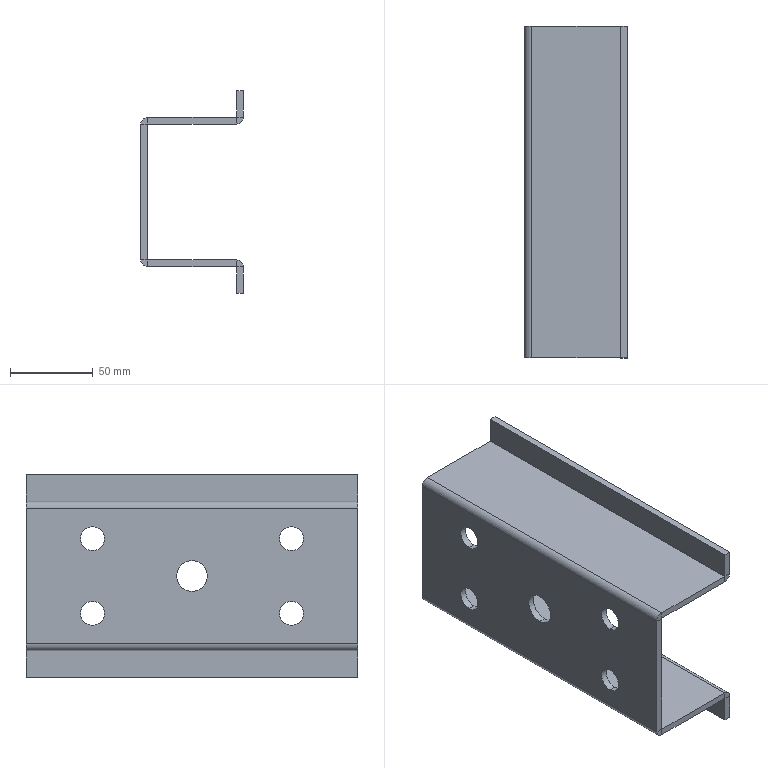Part | SolidWorks | features EdgeFlange 1, FlatPattern 1, ICE 1, SMBaseFlange 1, SheetMetal 1 | 1 solid | 48 faces | box 62 x 200 x 122 mm | volume 183661 mm3 | plane 30 | cylinder 18 | commonest cylinder face diameters 14.5 x8 0.4 x4 8.4 x4 18.5 x2
STEP:
#1=CARTESIAN_POINT('',(0.,0.,-9.25));
#2=VERTEX_POINT('',#1);
#3=CARTESIAN_POINT('',(0.,0.,9.25));
#4=VERTEX_POINT('',#3);
#5=CARTESIAN_POINT('',(0.,0.,0.));
#6=DIRECTION('',(-1.,0.,0.));
#7=DIRECTION('',(0.,0.,1.));
#8=AXIS2_PLACEMENT_3D('',#5,#6,#7);
#9=CIRCLE('',#8,9.25);
#10=EDGE_CURVE('',#2,#4,#9,.T.);
#11=ORIENTED_EDGE('',*,*,#10,.T.);
#12=CARTESIAN_POINT('',(4.,0.,9.25));
#13=VERTEX_POINT('',#12);
#14=CARTESIAN_POINT('',(-6.,0.,9.25));
#15=DIRECTION('',(1.,0.,0.));
#16=VECTOR('',#15,1000.);
#17=LINE('',#14,#16);
#18=EDGE_CURVE('',#4,#13,#17,.T.);
#19=ORIENTED_EDGE('',*,*,#18,.T.);
#20=CARTESIAN_POINT('',(4.,0.,-9.25));
#21=VERTEX_POINT('',#20);
#22=CARTESIAN_POINT('',(4.,0.,0.));
#23=DIRECTION('',(1.,0.,0.));
#24=DIRECTION('',(0.,0.,-1.));
#25=AXIS2_PLACEMENT_3D('',#22,#23,#24);
#26=CIRCLE('',#25,9.25);
#27=EDGE_CURVE('',#13,#21,#26,.T.);
#28=ORIENTED_EDGE('',*,*,#27,.T.);
#29=CARTESIAN_POINT('',(-6.,0.,-9.25));
#30=DIRECTION('',(1.,0.,0.));
#31=VECTOR('',#30,1000.);
#32=LINE('',#29,#31);
#33=EDGE_CURVE('',#2,#21,#32,.T.);
#34=ORIENTED_EDGE('',*,*,#33,.F.);
#35=EDGE_LOOP('',(#11,#19,#28,#34));
#36=FACE_OUTER_BOUND('',#35,.T.);
#37=CARTESIAN_POINT('',(-6.,0.,0.));
#38=DIRECTION('',(1.,0.,0.));
#39=DIRECTION('',(0.,0.,-1.));
#40=AXIS2_PLACEMENT_3D('',#37,#38,#39);
#41=CYLINDRICAL_SURFACE('',#40,9.25);
#42=ADVANCED_FACE('',(#36),#41,.F.);
#43=CARTESIAN_POINT('',(0.,-60.,-29.75));
#44=VERTEX_POINT('',#43);
#45=CARTESIAN_POINT('',(0.,-60.,-15.25));
#46=VERTEX_POINT('',#45);
#47=CARTESIAN_POINT('',(0.,-60.,-22.5));
#48=DIRECTION('',(-1.,0.,0.));
#49=DIRECTION('',(0.,0.,1.));
#50=AXIS2_PLACEMENT_3D('',#47,#48,#49);
#51=CIRCLE('',#50,7.25);
#52=EDGE_CURVE('',#44,#46,#51,.T.);
#53=ORIENTED_EDGE('',*,*,#52,.T.);
#54=CARTESIAN_POINT('',(4.,-60.,-15.25));
#55=VERTEX_POINT('',#54);
#56=CARTESIAN_POINT('',(-6.,-60.,-15.25));
#57=DIRECTION('',(1.,0.,0.));
#58=VECTOR('',#57,1000.);
#59=LINE('',#56,#58);
#60=EDGE_CURVE('',#46,#55,#59,.T.);
#61=ORIENTED_EDGE('',*,*,#60,.T.);
#62=CARTESIAN_POINT('',(4.,-60.,-29.75));
#63=VERTEX_POINT('',#62);
#64=CARTESIAN_POINT('',(4.,-60.,-22.5));
#65=DIRECTION('',(1.,0.,0.));
#66=DIRECTION('',(0.,0.,-1.));
#67=AXIS2_PLACEMENT_3D('',#64,#65,#66);
#68=CIRCLE('',#67,7.25);
#69=EDGE_CURVE('',#55,#63,#68,.T.);
#70=ORIENTED_EDGE('',*,*,#69,.T.);
#71=CARTESIAN_POINT('',(-6.,-60.,-29.75));
#72=DIRECTION('',(1.,0.,0.));
#73=VECTOR('',#72,1000.);
#74=LINE('',#71,#73);
#75=EDGE_CURVE('',#44,#63,#74,.T.);
#76=ORIENTED_EDGE('',*,*,#75,.F.);
#77=EDGE_LOOP('',(#53,#61,#70,#76));
#78=FACE_OUTER_BOUND('',#77,.T.);
#79=CARTESIAN_POINT('',(-6.,-60.,-22.5));
#80=DIRECTION('',(1.,0.,0.));
#81=DIRECTION('',(0.,0.,-1.));
#82=AXIS2_PLACEMENT_3D('',#79,#80,#81);
#83=CYLINDRICAL_SURFACE('',#82,7.25);
#84=ADVANCED_FACE('',(#78),#83,.F.);
#85=CARTESIAN_POINT('',(0.,-60.,15.25));
#86=VERTEX_POINT('',#85);
#87=CARTESIAN_POINT('',(0.,-60.,29.75));
#88=VERTEX_POINT('',#87);
#89=CARTESIAN_POINT('',(0.,-60.,22.5));
#90=DIRECTION('',(-1.,0.,0.));
#91=DIRECTION('',(0.,0.,1.));
#92=AXIS2_PLACEMENT_3D('',#89,#90,#91);
#93=CIRCLE('',#92,7.25);
#94=EDGE_CURVE('',#86,#88,#93,.T.);
#95=ORIENTED_EDGE('',*,*,#94,.T.);
#96=CARTESIAN_POINT('',(4.,-60.,29.75));
#97=VERTEX_POINT('',#96);
#98=CARTESIAN_POINT('',(-6.,-60.,29.75));
#99=DIRECTION('',(1.,0.,0.));
#100=VECTOR('',#99,1000.);
#101=LINE('',#98,#100);
#102=EDGE_CURVE('',#88,#97,#101,.T.);
#103=ORIENTED_EDGE('',*,*,#102,.T.);
#104=CARTESIAN_POINT('',(4.,-60.,15.25));
#105=VERTEX_POINT('',#104);
#106=CARTESIAN_POINT('',(4.,-60.,22.5));
#107=DIRECTION('',(1.,0.,0.));
#108=DIRECTION('',(0.,0.,-1.));
#109=AXIS2_PLACEMENT_3D('',#106,#107,#108);
#110=CIRCLE('',#109,7.25);
#111=EDGE_CURVE('',#97,#105,#110,.T.);
#112=ORIENTED_EDGE('',*,*,#111,.T.);
#113=CARTESIAN_POINT('',(-6.,-60.,15.25));
#114=DIRECTION('',(1.,0.,0.));
#115=VECTOR('',#114,1000.);
#116=LINE('',#113,#115);
#117=EDGE_CURVE('',#86,#105,#116,.T.);
#118=ORIENTED_EDGE('',*,*,#117,.F.);
#119=EDGE_LOOP('',(#95,#103,#112,#118));
#120=FACE_OUTER_BOUND('',#119,.T.);
#121=CARTESIAN_POINT('',(-6.,-60.,22.5));
#122=DIRECTION('',(1.,0.,0.));
#123=DIRECTION('',(0.,0.,-1.));
#124=AXIS2_PLACEMENT_3D('',#121,#122,#123);
#125=CYLINDRICAL_SURFACE('',#124,7.25);
#126=ADVANCED_FACE('',(#120),#125,.F.);
#127=CARTESIAN_POINT('',(0.,60.,15.25));
#128=VERTEX_POINT('',#127);
#129=CARTESIAN_POINT('',(0.,60.,29.75));
#130=VERTEX_POINT('',#129);
#131=CARTESIAN_POINT('',(0.,60.,22.5));
#132=DIRECTION('',(-1.,0.,0.));
#133=DIRECTION('',(0.,0.,1.));
#134=AXIS2_PLACEMENT_3D('',#131,#132,#133);
#135=CIRCLE('',#134,7.25);
#136=EDGE_CURVE('',#128,#130,#135,.T.);
#137=ORIENTED_EDGE('',*,*,#136,.T.);
#138=CARTESIAN_POINT('',(4.,60.,29.75));
#139=VERTEX_POINT('',#138);
#140=CARTESIAN_POINT('',(-6.,60.,29.75));
#141=DIRECTION('',(1.,0.,0.));
#142=VECTOR('',#141,1000.);
#143=LINE('',#140,#142);
#144=EDGE_CURVE('',#130,#139,#143,.T.);
#145=ORIENTED_EDGE('',*,*,#144,.T.);
#146=CARTESIAN_POINT('',(4.,60.,15.25));
#147=VERTEX_POINT('',#146);
#148=CARTESIAN_POINT('',(4.,60.,22.5));
#149=DIRECTION('',(1.,0.,0.));
#150=DIRECTION('',(0.,0.,-1.));
#151=AXIS2_PLACEMENT_3D('',#148,#149,#150);
#152=CIRCLE('',#151,7.25);
#153=EDGE_CURVE('',#139,#147,#152,.T.);
#154=ORIENTED_EDGE('',*,*,#153,.T.);
#155=CARTESIAN_POINT('',(-6.,60.,15.25));
#156=DIRECTION('',(1.,0.,0.));
#157=VECTOR('',#156,1000.);
#158=LINE('',#155,#157);
#159=EDGE_CURVE('',#128,#147,#158,.T.);
#160=ORIENTED_EDGE('',*,*,#159,.F.);
#161=EDGE_LOOP('',(#137,#145,#154,#160));
#162=FACE_OUTER_BOUND('',#161,.T.);
#163=CARTESIAN_POINT('',(-6.,60.,22.5));
#164=DIRECTION('',(1.,0.,0.));
#165=DIRECTION('',(0.,0.,-1.));
#166=AXIS2_PLACEMENT_3D('',#163,#164,#165);
#167=CYLINDRICAL_SURFACE('',#166,7.25);
#168=ADVANCED_FACE('',(#162),#167,.F.);
#169=CARTESIAN_POINT('',(0.,60.,-29.75));
#170=VERTEX_POINT('',#169);
#171=CARTESIAN_POINT('',(0.,60.,-15.25));
#172=VERTEX_POINT('',#171);
#173=CARTESIAN_POINT('',(0.,60.,-22.5));
#174=DIRECTION('',(-1.,0.,0.));
#175=DIRECTION('',(0.,0.,1.));
#176=AXIS2_PLACEMENT_3D('',#173,#174,#175);
#177=CIRCLE('',#176,7.25);
#178=EDGE_CURVE('',#170,#172,#177,.T.);
#179=ORIENTED_EDGE('',*,*,#178,.T.);
#180=CARTESIAN_POINT('',(4.,60.,-15.25));
#181=VERTEX_POINT('',#180);
#182=CARTESIAN_POINT('',(-6.,60.,-15.25));
#183=DIRECTION('',(1.,0.,0.));
#184=VECTOR('',#183,1000.);
#185=LINE('',#182,#184);
#186=EDGE_CURVE('',#172,#181,#185,.T.);
#187=ORIENTED_EDGE('',*,*,#186,.T.);
#188=CARTESIAN_POINT('',(4.,60.,-29.75));
#189=VERTEX_POINT('',#188);
#190=CARTESIAN_POINT('',(4.,60.,-22.5));
#191=DIRECTION('',(1.,0.,0.));
#192=DIRECTION('',(0.,0.,-1.));
#193=AXIS2_PLACEMENT_3D('',#190,#191,#192);
#194=CIRCLE('',#193,7.25);
#195=EDGE_CURVE('',#181,#189,#194,.T.);
#196=ORIENTED_EDGE('',*,*,#195,.T.);
#197=CARTESIAN_POINT('',(-6.,60.,-29.75));
#198=DIRECTION('',(1.,0.,0.));
#199=VECTOR('',#198,1000.);
#200=LINE('',#197,#199);
#201=EDGE_CURVE('',#170,#189,#200,.T.);
#202=ORIENTED_EDGE('',*,*,#201,.F.);
#203=EDGE_LOOP('',(#179,#187,#196,#202));
#204=FACE_OUTER_BOUND('',#203,.T.);
#205=CARTESIAN_POINT('',(-6.,60.,-22.5));
#206=DIRECTION('',(1.,0.,0.));
#207=DIRECTION('',(0.,0.,-1.));
#208=AXIS2_PLACEMENT_3D('',#205,#206,#207);
#209=CYLINDRICAL_SURFACE('',#208,7.25);
#210=ADVANCED_FACE('',(#204),#209,.F.);
#211=CARTESIAN_POINT('',(57.8,-100.,45.));
#212=VERTEX_POINT('',#211);
#213=CARTESIAN_POINT('',(4.2,-100.,45.));
#214=VERTEX_POINT('',#213);
#215=CARTESIAN_POINT('',(0.,-100.,45.));
#216=DIRECTION('',(-1.,0.,0.));
#217=VECTOR('',#216,1000.);
#218=LINE('',#215,#217);
#219=EDGE_CURVE('',#212,#214,#218,.T.);
#220=ORIENTED_EDGE('',*,*,#219,.F.);
#221=CARTESIAN_POINT('',(57.8,100.,45.));
#222=VERTEX_POINT('',#221);
#223=CARTESIAN_POINT('',(57.8,100.,45.));
#224=DIRECTION('',(0.,-1.,0.));
#225=VECTOR('',#224,1000.);
#226=LINE('',#223,#225);
#227=EDGE_CURVE('',#222,#212,#226,.T.);
#228=ORIENTED_EDGE('',*,*,#227,.F.);
#229=CARTESIAN_POINT('',(4.2,100.,45.));
#230=VERTEX_POINT('',#229);
#231=CARTESIAN_POINT('',(0.,100.,45.));
#232=DIRECTION('',(-1.,0.,0.));
#233=VECTOR('',#232,1000.);
#234=LINE('',#231,#233);
#235=EDGE_CURVE('',#222,#230,#234,.T.);
#236=ORIENTED_EDGE('',*,*,#235,.T.);
#237=CARTESIAN_POINT('',(4.2,100.,45.));
#238=DIRECTION('',(0.,-1.,0.));
#239=VECTOR('',#238,1000.);
#240=LINE('',#237,#239);
#241=EDGE_CURVE('',#230,#214,#240,.T.);
#242=ORIENTED_EDGE('',*,*,#241,.T.);
#243=EDGE_LOOP('',(#220,#228,#236,#242));
#244=FACE_OUTER_BOUND('',#243,.T.);
#245=CARTESIAN_POINT('',(0.,100.,45.));
#246=DIRECTION('',(0.,0.,1.));
#247=DIRECTION('',(1.,0.,0.));
#248=AXIS2_PLACEMENT_3D('',#245,#246,#247);
#249=PLANE('',#248);
#250=ADVANCED_FACE('',(#244),#249,.T.);
#251=CARTESIAN_POINT('',(57.8,100.,41.));
#252=VERTEX_POINT('',#251);
#253=CARTESIAN_POINT('',(57.8,-100.,41.));
#254=VERTEX_POINT('',#253);
#255=CARTESIAN_POINT('',(57.8,100.,41.));
#256=DIRECTION('',(0.,-1.,0.));
#257=VECTOR('',#256,1000.);
#258=LINE('',#255,#257);
#259=EDGE_CURVE('',#252,#254,#258,.T.);
#260=ORIENTED_EDGE('',*,*,#259,.T.);
#261=CARTESIAN_POINT('',(4.2,-100.,41.));
#262=VERTEX_POINT('',#261);
#263=CARTESIAN_POINT('',(0.,-100.,41.));
#264=DIRECTION('',(-1.,0.,0.));
#265=VECTOR('',#264,1000.);
#266=LINE('',#263,#265);
#267=EDGE_CURVE('',#254,#262,#266,.T.);
#268=ORIENTED_EDGE('',*,*,#267,.T.);
#269=CARTESIAN_POINT('',(4.2,100.,41.));
#270=VERTEX_POINT('',#269);
#271=CARTESIAN_POINT('',(4.2,100.,41.));
#272=DIRECTION('',(0.,-1.,0.));
#273=VECTOR('',#272,1000.);
#274=LINE('',#271,#273);
#275=EDGE_CURVE('',#270,#262,#274,.T.);
#276=ORIENTED_EDGE('',*,*,#275,.F.);
#277=CARTESIAN_POINT('',(0.,100.,41.));
#278=DIRECTION('',(-1.,0.,0.));
#279=VECTOR('',#278,1000.);
#280=LINE('',#277,#279);
#281=EDGE_CURVE('',#252,#270,#280,.T.);
#282=ORIENTED_EDGE('',*,*,#281,.F.);
#283=EDGE_LOOP('',(#260,#268,#276,#282));
#284=FACE_OUTER_BOUND('',#283,.T.);
#285=CARTESIAN_POINT('',(0.,100.,41.));
#286=DIRECTION('',(0.,0.,1.));
#287=DIRECTION('',(1.,0.,0.));
#288=AXIS2_PLACEMENT_3D('',#285,#286,#287);
#289=PLANE('',#288);
#290=ADVANCED_FACE('',(#284),#289,.F.);
#291=ORIENTED_EDGE('',*,*,#235,.F.);
#292=CARTESIAN_POINT('',(57.8,100.,45.));
#293=DIRECTION('',(0.,0.,-1.));
#294=VECTOR('',#293,1000.);
#295=LINE('',#292,#294);
#296=EDGE_CURVE('',#222,#252,#295,.T.);
#297=ORIENTED_EDGE('',*,*,#296,.T.);
#298=ORIENTED_EDGE('',*,*,#281,.T.);
#299=CARTESIAN_POINT('',(4.2,100.,41.));
#300=DIRECTION('',(0.,0.,1.));
#301=VECTOR('',#300,1000.);
#302=LINE('',#299,#301);
#303=EDGE_CURVE('',#270,#230,#302,.T.);
#304=ORIENTED_EDGE('',*,*,#303,.T.);
#305=EDGE_LOOP('',(#291,#297,#298,#304));
#306=FACE_OUTER_BOUND('',#305,.T.);
#307=CARTESIAN_POINT('',(4.2,100.,-40.8));
#308=DIRECTION('',(0.,1.,0.));
#309=DIRECTION('',(1.,0.,0.));
#310=AXIS2_PLACEMENT_3D('',#307,#308,#309);
#311=PLANE('',#310);
#312=ADVANCED_FACE('',(#306),#311,.T.);
#313=CARTESIAN_POINT('',(57.8,-100.,-41.));
#314=VERTEX_POINT('',#313);
#315=CARTESIAN_POINT('',(57.8,100.,-41.));
#316=VERTEX_POINT('',#315);
#317=CARTESIAN_POINT('',(57.8,-100.,-41.));
#318=DIRECTION('',(0.,1.,0.));
#319=VECTOR('',#318,1000.);
#320=LINE('',#317,#319);
#321=EDGE_CURVE('',#314,#316,#320,.T.);
#322=ORIENTED_EDGE('',*,*,#321,.T.);
#323=CARTESIAN_POINT('',(4.2,100.,-41.));
#324=VERTEX_POINT('',#323);
#325=CARTESIAN_POINT('',(0.,100.,-41.));
#326=DIRECTION('',(1.,0.,0.));
#327=VECTOR('',#326,1000.);
#328=LINE('',#325,#327);
#329=EDGE_CURVE('',#324,#316,#328,.T.);
#330=ORIENTED_EDGE('',*,*,#329,.F.);
#331=CARTESIAN_POINT('',(4.2,-100.,-41.));
#332=VERTEX_POINT('',#331);
#333=CARTESIAN_POINT('',(4.2,100.,-41.));
#334=DIRECTION('',(0.,-1.,0.));
#335=VECTOR('',#334,1000.);
#336=LINE('',#333,#335);
#337=EDGE_CURVE('',#324,#332,#336,.T.);
#338=ORIENTED_EDGE('',*,*,#337,.T.);
#339=CARTESIAN_POINT('',(0.,-100.,-41.));
#340=DIRECTION('',(1.,0.,0.));
#341=VECTOR('',#340,1000.);
#342=LINE('',#339,#341);
#343=EDGE_CURVE('',#332,#314,#342,.T.);
#344=ORIENTED_EDGE('',*,*,#343,.T.);
#345=EDGE_LOOP('',(#322,#330,#338,#344));
#346=FACE_OUTER_BOUND('',#345,.T.);
#347=CARTESIAN_POINT('',(0.,100.,-41.));
#348=DIRECTION('',(0.,0.,-1.));
#349=DIRECTION('',(-1.,0.,0.));
#350=AXIS2_PLACEMENT_3D('',#347,#348,#349);
#351=PLANE('',#350);
#352=ADVANCED_FACE('',(#346),#351,.F.);
#353=CARTESIAN_POINT('',(4.2,100.,-45.));
#354=VERTEX_POINT('',#353);
#355=CARTESIAN_POINT('',(57.8,100.,-45.));
#356=VERTEX_POINT('',#355);
#357=CARTESIAN_POINT('',(0.,100.,-45.));
#358=DIRECTION('',(1.,0.,0.));
#359=VECTOR('',#358,1000.);
#360=LINE('',#357,#359);
#361=EDGE_CURVE('',#354,#356,#360,.T.);
#362=ORIENTED_EDGE('',*,*,#361,.T.);
#363=CARTESIAN_POINT('',(57.8,-100.,-45.));
#364=VERTEX_POINT('',#363);
#365=CARTESIAN_POINT('',(57.8,-100.,-45.));
#366=DIRECTION('',(0.,1.,0.));
#367=VECTOR('',#366,1000.);
#368=LINE('',#365,#367);
#369=EDGE_CURVE('',#364,#356,#368,.T.);
#370=ORIENTED_EDGE('',*,*,#369,.F.);
#371=CARTESIAN_POINT('',(4.2,-100.,-45.));
#372=VERTEX_POINT('',#371);
#373=CARTESIAN_POINT('',(0.,-100.,-45.));
#374=DIRECTION('',(1.,0.,0.));
#375=VECTOR('',#374,1000.);
#376=LINE('',#373,#375);
#377=EDGE_CURVE('',#372,#364,#376,.T.);
#378=ORIENTED_EDGE('',*,*,#377,.F.);
#379=CARTESIAN_POINT('',(4.2,100.,-45.));
#380=DIRECTION('',(0.,-1.,0.));
#381=VECTOR('',#380,1000.);
#382=LINE('',#379,#381);
#383=EDGE_CURVE('',#354,#372,#382,.T.);
#384=ORIENTED_EDGE('',*,*,#383,.F.);
#385=EDGE_LOOP('',(#362,#370,#378,#384));
#386=FACE_OUTER_BOUND('',#385,.T.);
#387=CARTESIAN_POINT('',(0.,100.,-45.));
#388=DIRECTION('',(0.,0.,-1.));
#389=DIRECTION('',(-1.,0.,0.));
#390=AXIS2_PLACEMENT_3D('',#387,#388,#389);
#391=PLANE('',#390);
#392=ADVANCED_FACE('',(#386),#391,.T.);
#393=CARTESIAN_POINT('',(57.8,-100.,-45.));
#394=DIRECTION('',(0.,0.,1.));
#395=VECTOR('',#394,1000.);
#396=LINE('',#393,#395);
#397=EDGE_CURVE('',#364,#314,#396,.T.);
#398=ORIENTED_EDGE('',*,*,#397,.T.);
#399=ORIENTED_EDGE('',*,*,#343,.F.);
#400=CARTESIAN_POINT('',(4.2,-100.,-41.));
#401=DIRECTION('',(0.,0.,-1.));
#402=VECTOR('',#401,1000.);
#403=LINE('',#400,#402);
#404=EDGE_CURVE('',#332,#372,#403,.T.);
#405=ORIENTED_EDGE('',*,*,#404,.T.);
#406=ORIENTED_EDGE('',*,*,#377,.T.);
#407=EDGE_LOOP('',(#398,#399,#405,#406));
#408=FACE_OUTER_BOUND('',#407,.T.);
#409=CARTESIAN_POINT('',(4.2,-100.,-40.8));
#410=DIRECTION('',(0.,1.,0.));
#411=DIRECTION('',(1.,0.,0.));
#412=AXIS2_PLACEMENT_3D('',#409,#410,#411);
#413=PLANE('',#412);
#414=ADVANCED_FACE('',(#408),#413,.F.);
#415=CARTESIAN_POINT('',(0.,100.,40.8));
#416=VERTEX_POINT('',#415);
#417=CARTESIAN_POINT('',(4.,100.,40.8));
#418=VERTEX_POINT('',#417);
#419=CARTESIAN_POINT('',(0.,100.,40.8));
#420=DIRECTION('',(1.,0.,0.));
#421=VECTOR('',#420,1000.);
#422=LINE('',#419,#421);
#423=EDGE_CURVE('',#416,#418,#422,.T.);
#424=ORIENTED_EDGE('',*,*,#423,.F.);
#425=CARTESIAN_POINT('',(4.2,100.,40.8));
#426=DIRECTION('',(0.,-1.,0.));
#427=DIRECTION('',(0.,0.,1.));
#428=AXIS2_PLACEMENT_3D('',#425,#426,#427);
#429=CIRCLE('',#428,4.2);
#430=EDGE_CURVE('',#230,#416,#429,.T.);
#431=ORIENTED_EDGE('',*,*,#430,.F.);
#432=ORIENTED_EDGE('',*,*,#303,.F.);
#433=CARTESIAN_POINT('',(4.2,100.,40.8));
#434=DIRECTION('',(0.,-1.,0.));
#435=DIRECTION('',(1.,0.,0.));
#436=AXIS2_PLACEMENT_3D('',#433,#434,#435);
#437=CIRCLE('',#436,0.2);
#438=EDGE_CURVE('',#270,#418,#437,.T.);
#439=ORIENTED_EDGE('',*,*,#438,.T.);
#440=EDGE_LOOP('',(#424,#431,#432,#439));
#441=FACE_OUTER_BOUND('',#440,.T.);
#442=CARTESIAN_POINT('',(0.,100.,40.8));
#443=DIRECTION('',(0.,1.,0.));
#444=DIRECTION('',(0.,0.,1.));
#445=AXIS2_PLACEMENT_3D('',#442,#443,#444);
#446=PLANE('',#445);
#447=ADVANCED_FACE('',(#441),#446,.T.);
#448=CARTESIAN_POINT('',(0.,100.,-40.8));
#449=VERTEX_POINT('',#448);
#450=CARTESIAN_POINT('',(0.,100.,-45.));
#451=DIRECTION('',(0.,0.,-1.));
#452=VECTOR('',#451,1000.);
#453=LINE('',#450,#452);
#454=EDGE_CURVE('',#416,#449,#453,.T.);
#455=ORIENTED_EDGE('',*,*,#454,.F.);
#456=ORIENTED_EDGE('',*,*,#423,.T.);
#457=CARTESIAN_POINT('',(4.,100.,-40.8));
#458=VERTEX_POINT('',#457);
#459=CARTESIAN_POINT('',(4.,100.,-45.));
#460=DIRECTION('',(0.,0.,-1.));
#461=VECTOR('',#460,1000.);
#462=LINE('',#459,#461);
#463=EDGE_CURVE('',#418,#458,#462,.T.);
#464=ORIENTED_EDGE('',*,*,#463,.T.);
#465=CARTESIAN_POINT('',(4.,100.,-40.8));
#466=DIRECTION('',(-1.,0.,0.));
#467=VECTOR('',#466,1000.);
#468=LINE('',#465,#467);
#469=EDGE_CURVE('',#458,#449,#468,.T.);
#470=ORIENTED_EDGE('',*,*,#469,.T.);
#471=EDGE_LOOP('',(#455,#456,#464,#470));
#472=FACE_OUTER_BOUND('',#471,.T.);
#473=CARTESIAN_POINT('',(4.2,100.,41.));
#474=DIRECTION('',(0.,1.,0.));
#475=DIRECTION('',(0.,0.,1.));
#476=AXIS2_PLACEMENT_3D('',#473,#474,#475);
#477=PLANE('',#476);
#478=ADVANCED_FACE('',(#472),#477,.T.);
#479=CARTESIAN_POINT('',(4.2,-100.,45.));
#480=DIRECTION('',(0.,0.,-1.));
#481=VECTOR('',#480,1000.);
#482=LINE('',#479,#481);
#483=EDGE_CURVE('',#214,#262,#482,.T.);
#484=ORIENTED_EDGE('',*,*,#483,.F.);
#485=CARTESIAN_POINT('',(0.,-100.,40.8));
#486=VERTEX_POINT('',#485);
#487=CARTESIAN_POINT('',(4.2,-100.,40.8));
#488=DIRECTION('',(0.,-1.,0.));
#489=DIRECTION('',(0.,0.,1.));
#490=AXIS2_PLACEMENT_3D('',#487,#488,#489);
#491=CIRCLE('',#490,4.2);
#492=EDGE_CURVE('',#214,#486,#491,.T.);
#493=ORIENTED_EDGE('',*,*,#492,.T.);
#494=CARTESIAN_POINT('',(4.,-100.,40.8));
#495=VERTEX_POINT('',#494);
#496=CARTESIAN_POINT('',(4.,-100.,40.8));
#497=DIRECTION('',(-1.,0.,0.));
#498=VECTOR('',#497,1000.);
#499=LINE('',#496,#498);
#500=EDGE_CURVE('',#495,#486,#499,.T.);
#501=ORIENTED_EDGE('',*,*,#500,.F.);
#502=CARTESIAN_POINT('',(4.2,-100.,40.8));
#503=DIRECTION('',(0.,-1.,0.));
#504=DIRECTION('',(1.,0.,0.));
#505=AXIS2_PLACEMENT_3D('',#502,#503,#504);
#506=CIRCLE('',#505,0.2);
#507=EDGE_CURVE('',#262,#495,#506,.T.);
#508=ORIENTED_EDGE('',*,*,#507,.F.);
#509=EDGE_LOOP('',(#484,#493,#501,#508));
#510=FACE_OUTER_BOUND('',#509,.T.);
#511=CARTESIAN_POINT('',(4.2,-100.,45.));
#512=DIRECTION('',(0.,-1.,0.));
#513=DIRECTION('',(0.,0.,-1.));
#514=AXIS2_PLACEMENT_3D('',#511,#512,#513);
#515=PLANE('',#514);
#516=ADVANCED_FACE('',(#510),#515,.T.);
#517=CARTESIAN_POINT('',(57.8,-100.,45.));
#518=DIRECTION('',(0.,0.,-1.));
#519=VECTOR('',#518,1000.);
#520=LINE('',#517,#519);
#521=EDGE_CURVE('',#212,#254,#520,.T.);
#522=ORIENTED_EDGE('',*,*,#521,.F.);
#523=ORIENTED_EDGE('',*,*,#219,.T.);
#524=ORIENTED_EDGE('',*,*,#483,.T.);
#525=ORIENTED_EDGE('',*,*,#267,.F.);
#526=EDGE_LOOP('',(#522,#523,#524,#525));
#527=FACE_OUTER_BOUND('',#526,.T.);
#528=CARTESIAN_POINT('',(4.,-100.,40.8));
#529=DIRECTION('',(0.,-1.,0.));
#530=DIRECTION('',(0.,0.,-1.));
#531=AXIS2_PLACEMENT_3D('',#528,#529,#530);
#532=PLANE('',#531);
#533=ADVANCED_FACE('',(#527),#532,.T.);
#534=CARTESIAN_POINT('',(4.2,100.,-45.));
#535=DIRECTION('',(0.,0.,1.));
#536=VECTOR('',#535,1000.);
#537=LINE('',#534,#536);
#538=EDGE_CURVE('',#354,#324,#537,.T.);
#539=ORIENTED_EDGE('',*,*,#538,.F.);
#540=CARTESIAN_POINT('',(4.2,100.,-40.8));
#541=DIRECTION('',(0.,-1.,0.));
#542=DIRECTION('',(0.,0.,1.));
#543=AXIS2_PLACEMENT_3D('',#540,#541,#542);
#544=CIRCLE('',#543,4.2);
#545=EDGE_CURVE('',#449,#354,#544,.T.);
#546=ORIENTED_EDGE('',*,*,#545,.F.);
#547=ORIENTED_EDGE('',*,*,#469,.F.);
#548=CARTESIAN_POINT('',(4.2,100.,-40.8));
#549=DIRECTION('',(0.,-1.,0.));
#550=DIRECTION('',(1.,0.,0.));
#551=AXIS2_PLACEMENT_3D('',#548,#549,#550);
#552=CIRCLE('',#551,0.2);
#553=EDGE_CURVE('',#458,#324,#552,.T.);
#554=ORIENTED_EDGE('',*,*,#553,.T.);
#555=EDGE_LOOP('',(#539,#546,#547,#554));
#556=FACE_OUTER_BOUND('',#555,.T.);
#557=CARTESIAN_POINT('',(4.2,100.,-45.));
#558=DIRECTION('',(0.,1.,0.));
#559=DIRECTION('',(0.,0.,1.));
#560=AXIS2_PLACEMENT_3D('',#557,#558,#559);
#561=PLANE('',#560);
#562=ADVANCED_FACE('',(#556),#561,.T.);
#563=CARTESIAN_POINT('',(57.8,100.,-45.));
#564=DIRECTION('',(0.,0.,1.));
#565=VECTOR('',#564,1000.);
#566=LINE('',#563,#565);
#567=EDGE_CURVE('',#356,#316,#566,.T.);
#568=ORIENTED_EDGE('',*,*,#567,.F.);
#569=ORIENTED_EDGE('',*,*,#361,.F.);
#570=ORIENTED_EDGE('',*,*,#538,.T.);
#571=ORIENTED_EDGE('',*,*,#329,.T.);
#572=EDGE_LOOP('',(#568,#569,#570,#571));
#573=FACE_OUTER_BOUND('',#572,.T.);
#574=CARTESIAN_POINT('',(4.,100.,-40.8));
#575=DIRECTION('',(0.,1.,0.));
#576=DIRECTION('',(0.,0.,1.));
#577=AXIS2_PLACEMENT_3D('',#574,#575,#576);
#578=PLANE('',#577);
#579=ADVANCED_FACE('',(#573),#578,.T.);
#580=CARTESIAN_POINT('',(0.,-100.,-40.8));
#581=VERTEX_POINT('',#580);
#582=CARTESIAN_POINT('',(4.,-100.,-40.8));
#583=VERTEX_POINT('',#582);
#584=CARTESIAN_POINT('',(0.,-100.,-40.8));
#585=DIRECTION('',(1.,0.,0.));
#586=VECTOR('',#585,1000.);
#587=LINE('',#584,#586);
#588=EDGE_CURVE('',#581,#583,#587,.T.);
#589=ORIENTED_EDGE('',*,*,#588,.F.);
#590=CARTESIAN_POINT('',(4.2,-100.,-40.8));
#591=DIRECTION('',(0.,-1.,0.));
#592=DIRECTION('',(0.,0.,1.));
#593=AXIS2_PLACEMENT_3D('',#590,#591,#592);
#594=CIRCLE('',#593,4.2);
#595=EDGE_CURVE('',#581,#372,#594,.T.);
#596=ORIENTED_EDGE('',*,*,#595,.T.);
#597=ORIENTED_EDGE('',*,*,#404,.F.);
#598=CARTESIAN_POINT('',(4.2,-100.,-40.8));
#599=DIRECTION('',(0.,-1.,0.));
#600=DIRECTION('',(1.,0.,0.));
#601=AXIS2_PLACEMENT_3D('',#598,#599,#600);
#602=CIRCLE('',#601,0.2);
#603=EDGE_CURVE('',#583,#332,#602,.T.);
#604=ORIENTED_EDGE('',*,*,#603,.F.);
#605=EDGE_LOOP('',(#589,#596,#597,#604));
#606=FACE_OUTER_BOUND('',#605,.T.);
#607=CARTESIAN_POINT('',(0.,-100.,-40.8));
#608=DIRECTION('',(0.,-1.,0.));
#609=DIRECTION('',(0.,0.,-1.));
#610=AXIS2_PLACEMENT_3D('',#607,#608,#609);
#611=PLANE('',#610);
#612=ADVANCED_FACE('',(#606),#611,.T.);
#613=CARTESIAN_POINT('',(0.,-100.,-45.));
#614=DIRECTION('',(0.,0.,-1.));
#615=VECTOR('',#614,1000.);
#616=LINE('',#613,#615);
#617=EDGE_CURVE('',#486,#581,#616,.T.);
#618=ORIENTED_EDGE('',*,*,#617,.T.);
#619=ORIENTED_EDGE('',*,*,#588,.T.);
#620=CARTESIAN_POINT('',(4.,-100.,-45.));
#621=DIRECTION('',(0.,0.,-1.));
#622=VECTOR('',#621,1000.);
#623=LINE('',#620,#622);
#624=EDGE_CURVE('',#495,#583,#623,.T.);
#625=ORIENTED_EDGE('',*,*,#624,.F.);
#626=ORIENTED_EDGE('',*,*,#500,.T.);
#627=EDGE_LOOP('',(#618,#619,#625,#626));
#628=FACE_OUTER_BOUND('',#627,.T.);
#629=CARTESIAN_POINT('',(4.2,-100.,-41.));
#630=DIRECTION('',(0.,-1.,0.));
#631=DIRECTION('',(0.,0.,-1.));
#632=AXIS2_PLACEMENT_3D('',#629,#630,#631);
#633=PLANE('',#632);
#634=ADVANCED_FACE('',(#628),#633,.T.);
#635=ORIENTED_EDGE('',*,*,#595,.F.);
#636=CARTESIAN_POINT('',(0.,100.,-40.8));
#637=DIRECTION('',(0.,-1.,0.));
#638=VECTOR('',#637,1000.);
#639=LINE('',#636,#638);
#640=EDGE_CURVE('',#449,#581,#639,.T.);
#641=ORIENTED_EDGE('',*,*,#640,.F.);
#642=ORIENTED_EDGE('',*,*,#545,.T.);
#643=ORIENTED_EDGE('',*,*,#383,.T.);
#644=EDGE_LOOP('',(#635,#641,#642,#643));
#645=FACE_OUTER_BOUND('',#644,.T.);
#646=CARTESIAN_POINT('',(4.2,100.,-40.8));
#647=DIRECTION('',(0.,-1.,0.));
#648=DIRECTION('',(0.,0.,-1.));
#649=AXIS2_PLACEMENT_3D('',#646,#647,#648);
#650=CYLINDRICAL_SURFACE('',#649,4.2);
#651=ADVANCED_FACE('',(#645),#650,.T.);
#652=ORIENTED_EDGE('',*,*,#10,.F.);
#653=CARTESIAN_POINT('',(0.,0.,0.));
#654=DIRECTION('',(-1.,0.,0.));
#655=DIRECTION('',(0.,0.,1.));
#656=AXIS2_PLACEMENT_3D('',#653,#654,#655);
#657=CIRCLE('',#656,9.25);
#658=EDGE_CURVE('',#4,#2,#657,.T.);
#659=ORIENTED_EDGE('',*,*,#658,.F.);
#660=EDGE_LOOP('',(#652,#659));
#661=FACE_BOUND('',#660,.T.);
#662=ORIENTED_EDGE('',*,*,#52,.F.);
#663=CARTESIAN_POINT('',(0.,-60.,-22.5));
#664=DIRECTION('',(-1.,0.,0.));
#665=DIRECTION('',(0.,0.,1.));
#666=AXIS2_PLACEMENT_3D('',#663,#664,#665);
#667=CIRCLE('',#666,7.25);
#668=EDGE_CURVE('',#46,#44,#667,.T.);
#669=ORIENTED_EDGE('',*,*,#668,.F.);
#670=EDGE_LOOP('',(#662,#669));
#671=FACE_BOUND('',#670,.T.);
#672=ORIENTED_EDGE('',*,*,#94,.F.);
#673=CARTESIAN_POINT('',(0.,-60.,22.5));
#674=DIRECTION('',(-1.,0.,0.));
#675=DIRECTION('',(0.,0.,1.));
#676=AXIS2_PLACEMENT_3D('',#673,#674,#675);
#677=CIRCLE('',#676,7.25);
#678=EDGE_CURVE('',#88,#86,#677,.T.);
#679=ORIENTED_EDGE('',*,*,#678,.F.);
#680=EDGE_LOOP('',(#672,#679));
#681=FACE_BOUND('',#680,.T.);
#682=ORIENTED_EDGE('',*,*,#136,.F.);
#683=CARTESIAN_POINT('',(0.,60.,22.5));
#684=DIRECTION('',(-1.,0.,0.));
#685=DIRECTION('',(0.,0.,1.));
#686=AXIS2_PLACEMENT_3D('',#683,#684,#685);
#687=CIRCLE('',#686,7.25);
#688=EDGE_CURVE('',#130,#128,#687,.T.);
#689=ORIENTED_EDGE('',*,*,#688,.F.);
#690=EDGE_LOOP('',(#682,#689));
#691=FACE_BOUND('',#690,.T.);
#692=ORIENTED_EDGE('',*,*,#178,.F.);
#693=CARTESIAN_POINT('',(0.,60.,-22.5));
#694=DIRECTION('',(-1.,0.,0.));
#695=DIRECTION('',(0.,0.,1.));
#696=AXIS2_PLACEMENT_3D('',#693,#694,#695);
#697=CIRCLE('',#696,7.25);
#698=EDGE_CURVE('',#172,#170,#697,.T.);
#699=ORIENTED_EDGE('',*,*,#698,.F.);
#700=EDGE_LOOP('',(#692,#699));
#701=FACE_BOUND('',#700,.T.);
#702=ORIENTED_EDGE('',*,*,#617,.F.);
#703=CARTESIAN_POINT('',(0.,100.,40.8));
#704=DIRECTION('',(0.,-1.,0.));
#705=VECTOR('',#704,1000.);
#706=LINE('',#703,#705);
#707=EDGE_CURVE('',#416,#486,#706,.T.);
#708=ORIENTED_EDGE('',*,*,#707,.F.);
#709=ORIENTED_EDGE('',*,*,#454,.T.);
#710=ORIENTED_EDGE('',*,*,#640,.T.);
#711=EDGE_LOOP('',(#702,#708,#709,#710));
#712=FACE_OUTER_BOUND('',#711,.T.);
#713=CARTESIAN_POINT('',(0.,100.,-45.));
#714=DIRECTION('',(-1.,0.,0.));
#715=DIRECTION('',(0.,0.,1.));
#716=AXIS2_PLACEMENT_3D('',#713,#714,#715);
#717=PLANE('',#716);
#718=ADVANCED_FACE('',(#661,#671,#681,#691,#701,#712),#717,.T.);
#719=ORIENTED_EDGE('',*,*,#492,.F.);
#720=ORIENTED_EDGE('',*,*,#241,.F.);
#721=ORIENTED_EDGE('',*,*,#430,.T.);
#722=ORIENTED_EDGE('',*,*,#707,.T.);
#723=EDGE_LOOP('',(#719,#720,#721,#722));
#724=FACE_OUTER_BOUND('',#723,.T.);
#725=CARTESIAN_POINT('',(4.2,100.,40.8));
#726=DIRECTION('',(0.,-1.,0.));
#727=DIRECTION('',(0.,0.,-1.));
#728=AXIS2_PLACEMENT_3D('',#725,#726,#727);
#729=CYLINDRICAL_SURFACE('',#728,4.2);
#730=ADVANCED_FACE('',(#724),#729,.T.);
#731=ORIENTED_EDGE('',*,*,#507,.T.);
#732=CARTESIAN_POINT('',(4.,100.,40.8));
#733=DIRECTION('',(0.,-1.,0.));
#734=VECTOR('',#733,1000.);
#735=LINE('',#732,#734);
#736=EDGE_CURVE('',#418,#495,#735,.T.);
#737=ORIENTED_EDGE('',*,*,#736,.F.);
#738=ORIENTED_EDGE('',*,*,#438,.F.);
#739=ORIENTED_EDGE('',*,*,#275,.T.);
#740=EDGE_LOOP('',(#731,#737,#738,#739));
#741=FACE_OUTER_BOUND('',#740,.T.);
#742=CARTESIAN_POINT('',(4.2,100.,40.8));
#743=DIRECTION('',(0.,-1.,0.));
#744=DIRECTION('',(0.,0.,-1.));
#745=AXIS2_PLACEMENT_3D('',#742,#743,#744);
#746=CYLINDRICAL_SURFACE('',#745,0.2);
#747=ADVANCED_FACE('',(#741),#746,.F.);
#748=CARTESIAN_POINT('',(4.,0.,0.));
#749=DIRECTION('',(1.,0.,0.));
#750=DIRECTION('',(0.,0.,-1.));
#751=AXIS2_PLACEMENT_3D('',#748,#749,#750);
#752=CIRCLE('',#751,9.25);
#753=EDGE_CURVE('',#21,#13,#752,.T.);
#754=ORIENTED_EDGE('',*,*,#753,.F.);
#755=ORIENTED_EDGE('',*,*,#27,.F.);
#756=EDGE_LOOP('',(#754,#755));
#757=FACE_BOUND('',#756,.T.);
#758=CARTESIAN_POINT('',(4.,-60.,-22.5));
#759=DIRECTION('',(1.,0.,0.));
#760=DIRECTION('',(0.,0.,-1.));
#761=AXIS2_PLACEMENT_3D('',#758,#759,#760);
#762=CIRCLE('',#761,7.25);
#763=EDGE_CURVE('',#63,#55,#762,.T.);
#764=ORIENTED_EDGE('',*,*,#763,.F.);
#765=ORIENTED_EDGE('',*,*,#69,.F.);
#766=EDGE_LOOP('',(#764,#765));
#767=FACE_BOUND('',#766,.T.);
#768=CARTESIAN_POINT('',(4.,-60.,22.5));
#769=DIRECTION('',(1.,0.,0.));
#770=DIRECTION('',(0.,0.,-1.));
#771=AXIS2_PLACEMENT_3D('',#768,#769,#770);
#772=CIRCLE('',#771,7.25);
#773=EDGE_CURVE('',#105,#97,#772,.T.);
#774=ORIENTED_EDGE('',*,*,#773,.F.);
#775=ORIENTED_EDGE('',*,*,#111,.F.);
#776=EDGE_LOOP('',(#774,#775));
#777=FACE_BOUND('',#776,.T.);
#778=CARTESIAN_POINT('',(4.,60.,22.5));
#779=DIRECTION('',(1.,0.,0.));
#780=DIRECTION('',(0.,0.,-1.));
#781=AXIS2_PLACEMENT_3D('',#778,#779,#780);
#782=CIRCLE('',#781,7.25);
#783=EDGE_CURVE('',#147,#139,#782,.T.);
#784=ORIENTED_EDGE('',*,*,#783,.F.);
#785=ORIENTED_EDGE('',*,*,#153,.F.);
#786=EDGE_LOOP('',(#784,#785));
#787=FACE_BOUND('',#786,.T.);
#788=CARTESIAN_POINT('',(4.,60.,-22.5));
#789=DIRECTION('',(1.,0.,0.));
#790=DIRECTION('',(0.,0.,-1.));
#791=AXIS2_PLACEMENT_3D('',#788,#789,#790);
#792=CIRCLE('',#791,7.25);
#793=EDGE_CURVE('',#189,#181,#792,.T.);
#794=ORIENTED_EDGE('',*,*,#793,.F.);
#795=ORIENTED_EDGE('',*,*,#195,.F.);
#796=EDGE_LOOP('',(#794,#795));
#797=FACE_BOUND('',#796,.T.);
#798=ORIENTED_EDGE('',*,*,#624,.T.);
#799=CARTESIAN_POINT('',(4.,100.,-40.8));
#800=DIRECTION('',(0.,-1.,0.));
#801=VECTOR('',#800,1000.);
#802=LINE('',#799,#801);
#803=EDGE_CURVE('',#458,#583,#802,.T.);
#804=ORIENTED_EDGE('',*,*,#803,.F.);
#805=ORIENTED_EDGE('',*,*,#463,.F.);
#806=ORIENTED_EDGE('',*,*,#736,.T.);
#807=EDGE_LOOP('',(#798,#804,#805,#806));
#808=FACE_OUTER_BOUND('',#807,.T.);
#809=CARTESIAN_POINT('',(4.,100.,-45.));
#810=DIRECTION('',(-1.,0.,0.));
#811=DIRECTION('',(0.,0.,1.));
#812=AXIS2_PLACEMENT_3D('',#809,#810,#811);
#813=PLANE('',#812);
#814=ADVANCED_FACE('',(#757,#767,#777,#787,#797,#808),#813,.F.);
#815=ORIENTED_EDGE('',*,*,#603,.T.);
#816=ORIENTED_EDGE('',*,*,#337,.F.);
#817=ORIENTED_EDGE('',*,*,#553,.F.);
#818=ORIENTED_EDGE('',*,*,#803,.T.);
#819=EDGE_LOOP('',(#815,#816,#817,#818));
#820=FACE_OUTER_BOUND('',#819,.T.);
#821=CARTESIAN_POINT('',(4.2,100.,-40.8));
#822=DIRECTION('',(0.,-1.,0.));
#823=DIRECTION('',(0.,0.,-1.));
#824=AXIS2_PLACEMENT_3D('',#821,#822,#823);
#825=CYLINDRICAL_SURFACE('',#824,0.2);
#826=ADVANCED_FACE('',(#820),#825,.F.);
#827=CARTESIAN_POINT('',(58.,100.,-45.2));
#828=VERTEX_POINT('',#827);
#829=CARTESIAN_POINT('',(62.,100.,-45.2));
#830=VERTEX_POINT('',#829);
#831=CARTESIAN_POINT('',(62.,100.,-45.2));
#832=DIRECTION('',(1.,0.,0.));
#833=VECTOR('',#832,1000.);
#834=LINE('',#831,#833);
#835=EDGE_CURVE('',#828,#830,#834,.T.);
#836=ORIENTED_EDGE('',*,*,#835,.F.);
#837=CARTESIAN_POINT('',(57.8,100.,-45.2));
#838=DIRECTION('',(0.,1.,0.));
#839=DIRECTION('',(0.,0.,-1.));
#840=AXIS2_PLACEMENT_3D('',#837,#838,#839);
#841=CIRCLE('',#840,0.2);
#842=EDGE_CURVE('',#356,#828,#841,.T.);
#843=ORIENTED_EDGE('',*,*,#842,.F.);
#844=ORIENTED_EDGE('',*,*,#567,.T.);
#845=CARTESIAN_POINT('',(57.8,100.,-45.2));
#846=DIRECTION('',(0.,1.,0.));
#847=DIRECTION('',(0.,0.,-1.));
#848=AXIS2_PLACEMENT_3D('',#845,#846,#847);
#849=CIRCLE('',#848,4.2);
#850=EDGE_CURVE('',#316,#830,#849,.T.);
#851=ORIENTED_EDGE('',*,*,#850,.T.);
#852=EDGE_LOOP('',(#836,#843,#844,#851));
#853=FACE_OUTER_BOUND('',#852,.T.);
#854=CARTESIAN_POINT('',(57.8,100.,-45.2));
#855=DIRECTION('',(0.,1.,0.));
#856=DIRECTION('',(0.,0.,1.));
#857=AXIS2_PLACEMENT_3D('',#854,#855,#856);
#858=PLANE('',#857);
#859=ADVANCED_FACE('',(#853),#858,.T.);
#860=CARTESIAN_POINT('',(58.,-100.,-45.2));
#861=VERTEX_POINT('',#860);
#862=CARTESIAN_POINT('',(57.8,-100.,-45.2));
#863=DIRECTION('',(0.,-1.,0.));
#864=DIRECTION('',(0.,0.,-1.));
#865=AXIS2_PLACEMENT_3D('',#862,#863,#864);
#866=CIRCLE('',#865,0.2);
#867=EDGE_CURVE('',#861,#364,#866,.T.);
#868=ORIENTED_EDGE('',*,*,#867,.F.);
#869=CARTESIAN_POINT('',(62.,-100.,-45.2));
#870=VERTEX_POINT('',#869);
#871=CARTESIAN_POINT('',(58.,-100.,-45.2));
#872=DIRECTION('',(1.,0.,0.));
#873=VECTOR('',#872,1000.);
#874=LINE('',#871,#873);
#875=EDGE_CURVE('',#861,#870,#874,.T.);
#876=ORIENTED_EDGE('',*,*,#875,.T.);
#877=CARTESIAN_POINT('',(57.8,-100.,-45.2));
#878=DIRECTION('',(0.,-1.,0.));
#879=DIRECTION('',(0.,0.,-1.));
#880=AXIS2_PLACEMENT_3D('',#877,#878,#879);
#881=CIRCLE('',#880,4.2);
#882=EDGE_CURVE('',#870,#314,#881,.T.);
#883=ORIENTED_EDGE('',*,*,#882,.T.);
#884=ORIENTED_EDGE('',*,*,#397,.F.);
#885=EDGE_LOOP('',(#868,#876,#883,#884));
#886=FACE_OUTER_BOUND('',#885,.T.);
#887=CARTESIAN_POINT('',(57.8,-100.,-45.2));
#888=DIRECTION('',(0.,1.,0.));
#889=DIRECTION('',(0.,0.,1.));
#890=AXIS2_PLACEMENT_3D('',#887,#888,#889);
#891=PLANE('',#890);
#892=ADVANCED_FACE('',(#886),#891,.F.);
#893=ORIENTED_EDGE('',*,*,#321,.F.);
#894=ORIENTED_EDGE('',*,*,#882,.F.);
#895=CARTESIAN_POINT('',(62.,100.,-45.2));
#896=DIRECTION('',(0.,1.,0.));
#897=VECTOR('',#896,1000.);
#898=LINE('',#895,#897);
#899=EDGE_CURVE('',#870,#830,#898,.T.);
#900=ORIENTED_EDGE('',*,*,#899,.T.);
#901=ORIENTED_EDGE('',*,*,#850,.F.);
#902=EDGE_LOOP('',(#893,#894,#900,#901));
#903=FACE_OUTER_BOUND('',#902,.T.);
#904=CARTESIAN_POINT('',(57.8,-100.,-45.2));
#905=DIRECTION('',(0.,-1.,0.));
#906=DIRECTION('',(1.,0.,0.));
#907=AXIS2_PLACEMENT_3D('',#904,#905,#906);
#908=CYLINDRICAL_SURFACE('',#907,4.2);
#909=ADVANCED_FACE('',(#903),#908,.T.);
#910=ORIENTED_EDGE('',*,*,#369,.T.);
#911=ORIENTED_EDGE('',*,*,#842,.T.);
#912=CARTESIAN_POINT('',(58.,100.,-45.2));
#913=DIRECTION('',(0.,-1.,0.));
#914=VECTOR('',#913,1000.);
#915=LINE('',#912,#914);
#916=EDGE_CURVE('',#828,#861,#915,.T.);
#917=ORIENTED_EDGE('',*,*,#916,.T.);
#918=ORIENTED_EDGE('',*,*,#867,.T.);
#919=EDGE_LOOP('',(#910,#911,#917,#918));
#920=FACE_OUTER_BOUND('',#919,.T.);
#921=CARTESIAN_POINT('',(57.8,-100.,-45.2));
#922=DIRECTION('',(0.,-1.,0.));
#923=DIRECTION('',(1.,0.,0.));
#924=AXIS2_PLACEMENT_3D('',#921,#922,#923);
#925=CYLINDRICAL_SURFACE('',#924,0.2);
#926=ADVANCED_FACE('',(#920),#925,.F.);
#927=ORIENTED_EDGE('',*,*,#875,.F.);
#928=CARTESIAN_POINT('',(58.,-100.,-61.));
#929=VERTEX_POINT('',#928);
#930=CARTESIAN_POINT('',(58.,-100.,-61.));
#931=DIRECTION('',(0.,0.,-1.));
#932=VECTOR('',#931,1000.);
#933=LINE('',#930,#932);
#934=EDGE_CURVE('',#861,#929,#933,.T.);
#935=ORIENTED_EDGE('',*,*,#934,.T.);
#936=CARTESIAN_POINT('',(62.,-100.,-61.));
#937=VERTEX_POINT('',#936);
#938=CARTESIAN_POINT('',(62.,-100.,-61.));
#939=DIRECTION('',(-1.,0.,0.));
#940=VECTOR('',#939,1000.);
#941=LINE('',#938,#940);
#942=EDGE_CURVE('',#937,#929,#941,.T.);
#943=ORIENTED_EDGE('',*,*,#942,.F.);
#944=CARTESIAN_POINT('',(62.,-100.,0.));
#945=DIRECTION('',(0.,0.,-1.));
#946=VECTOR('',#945,1000.);
#947=LINE('',#944,#946);
#948=EDGE_CURVE('',#870,#937,#947,.T.);
#949=ORIENTED_EDGE('',*,*,#948,.F.);
#950=EDGE_LOOP('',(#927,#935,#943,#949));
#951=FACE_OUTER_BOUND('',#950,.T.);
#952=CARTESIAN_POINT('',(62.,-100.,-61.));
#953=DIRECTION('',(0.,1.,0.));
#954=DIRECTION('',(0.,0.,1.));
#955=AXIS2_PLACEMENT_3D('',#952,#953,#954);
#956=PLANE('',#955);
#957=ADVANCED_FACE('',(#951),#956,.F.);
#958=ORIENTED_EDGE('',*,*,#835,.T.);
#959=CARTESIAN_POINT('',(62.,100.,-61.));
#960=VERTEX_POINT('',#959);
#961=CARTESIAN_POINT('',(62.,100.,0.));
#962=DIRECTION('',(0.,0.,1.));
#963=VECTOR('',#962,1000.);
#964=LINE('',#961,#963);
#965=EDGE_CURVE('',#960,#830,#964,.T.);
#966=ORIENTED_EDGE('',*,*,#965,.F.);
#967=CARTESIAN_POINT('',(58.,100.,-61.));
#968=VERTEX_POINT('',#967);
#969=CARTESIAN_POINT('',(62.,100.,-61.));
#970=DIRECTION('',(-1.,0.,0.));
#971=VECTOR('',#970,1000.);
#972=LINE('',#969,#971);
#973=EDGE_CURVE('',#960,#968,#972,.T.);
#974=ORIENTED_EDGE('',*,*,#973,.T.);
#975=CARTESIAN_POINT('',(58.,100.,-45.));
#976=DIRECTION('',(0.,0.,1.));
#977=VECTOR('',#976,1000.);
#978=LINE('',#975,#977);
#979=EDGE_CURVE('',#968,#828,#978,.T.);
#980=ORIENTED_EDGE('',*,*,#979,.T.);
#981=EDGE_LOOP('',(#958,#966,#974,#980));
#982=FACE_OUTER_BOUND('',#981,.T.);
#983=CARTESIAN_POINT('',(62.,100.,-45.));
#984=DIRECTION('',(0.,-1.,0.));
#985=DIRECTION('',(0.,0.,-1.));
#986=AXIS2_PLACEMENT_3D('',#983,#984,#985);
#987=PLANE('',#986);
#988=ADVANCED_FACE('',(#982),#987,.F.);
#989=ORIENTED_EDGE('',*,*,#899,.F.);
#990=ORIENTED_EDGE('',*,*,#948,.T.);
#991=CARTESIAN_POINT('',(62.,0.,-61.));
#992=DIRECTION('',(0.,1.,0.));
#993=VECTOR('',#992,1000.);
#994=LINE('',#991,#993);
#995=EDGE_CURVE('',#937,#960,#994,.T.);
#996=ORIENTED_EDGE('',*,*,#995,.T.);
#997=ORIENTED_EDGE('',*,*,#965,.T.);
#998=EDGE_LOOP('',(#989,#990,#996,#997));
#999=FACE_OUTER_BOUND('',#998,.T.);
#1000=CARTESIAN_POINT('',(62.,0.,0.));
#1001=DIRECTION('',(-1.,0.,0.));
#1002=DIRECTION('',(0.,0.,1.));
#1003=AXIS2_PLACEMENT_3D('',#1000,#1001,#1002);
#1004=PLANE('',#1003);
#1005=ADVANCED_FACE('',(#999),#1004,.F.);
#1006=ORIENTED_EDGE('',*,*,#934,.F.);
#1007=ORIENTED_EDGE('',*,*,#916,.F.);
#1008=ORIENTED_EDGE('',*,*,#979,.F.);
#1009=CARTESIAN_POINT('',(58.,100.,-61.));
#1010=DIRECTION('',(0.,1.,0.));
#1011=VECTOR('',#1010,1000.);
#1012=LINE('',#1009,#1011);
#1013=EDGE_CURVE('',#929,#968,#1012,.T.);
#1014=ORIENTED_EDGE('',*,*,#1013,.F.);
#1015=EDGE_LOOP('',(#1006,#1007,#1008,#1014));
#1016=FACE_OUTER_BOUND('',#1015,.T.);
#1017=CARTESIAN_POINT('',(58.,0.,0.));
#1018=DIRECTION('',(-1.,0.,0.));
#1019=DIRECTION('',(0.,0.,1.));
#1020=AXIS2_PLACEMENT_3D('',#1017,#1018,#1019);
#1021=PLANE('',#1020);
#1022=ADVANCED_FACE('',(#1016),#1021,.T.);
#1023=ORIENTED_EDGE('',*,*,#1013,.T.);
#1024=ORIENTED_EDGE('',*,*,#973,.F.);
#1025=ORIENTED_EDGE('',*,*,#995,.F.);
#1026=ORIENTED_EDGE('',*,*,#942,.T.);
#1027=EDGE_LOOP('',(#1023,#1024,#1025,#1026));
#1028=FACE_OUTER_BOUND('',#1027,.T.);
#1029=CARTESIAN_POINT('',(62.,100.,-61.));
#1030=DIRECTION('',(0.,0.,1.));
#1031=DIRECTION('',(1.,0.,0.));
#1032=AXIS2_PLACEMENT_3D('',#1029,#1030,#1031);
#1033=PLANE('',#1032);
#1034=ADVANCED_FACE('',(#1028),#1033,.F.);
#1035=CARTESIAN_POINT('',(58.,-100.,45.2));
#1036=VERTEX_POINT('',#1035);
#1037=CARTESIAN_POINT('',(62.,-100.,45.2));
#1038=VERTEX_POINT('',#1037);
#1039=CARTESIAN_POINT('',(62.,-100.,45.2));
#1040=DIRECTION('',(1.,0.,0.));
#1041=VECTOR('',#1040,1000.);
#1042=LINE('',#1039,#1041);
#1043=EDGE_CURVE('',#1036,#1038,#1042,.T.);
#1044=ORIENTED_EDGE('',*,*,#1043,.F.);
#1045=CARTESIAN_POINT('',(57.8,-100.,45.2));
#1046=DIRECTION('',(0.,-1.,0.));
#1047=DIRECTION('',(0.,0.,1.));
#1048=AXIS2_PLACEMENT_3D('',#1045,#1046,#1047);
#1049=CIRCLE('',#1048,0.2);
#1050=EDGE_CURVE('',#212,#1036,#1049,.T.);
#1051=ORIENTED_EDGE('',*,*,#1050,.F.);
#1052=ORIENTED_EDGE('',*,*,#521,.T.);
#1053=CARTESIAN_POINT('',(57.8,-100.,45.2));
#1054=DIRECTION('',(0.,-1.,0.));
#1055=DIRECTION('',(0.,0.,1.));
#1056=AXIS2_PLACEMENT_3D('',#1053,#1054,#1055);
#1057=CIRCLE('',#1056,4.2);
#1058=EDGE_CURVE('',#254,#1038,#1057,.T.);
#1059=ORIENTED_EDGE('',*,*,#1058,.T.);
#1060=EDGE_LOOP('',(#1044,#1051,#1052,#1059));
#1061=FACE_OUTER_BOUND('',#1060,.T.);
#1062=CARTESIAN_POINT('',(57.8,-100.,45.2));
#1063=DIRECTION('',(0.,-1.,0.));
#1064=DIRECTION('',(0.,0.,-1.));
#1065=AXIS2_PLACEMENT_3D('',#1062,#1063,#1064);
#1066=PLANE('',#1065);
#1067=ADVANCED_FACE('',(#1061),#1066,.T.);
#1068=CARTESIAN_POINT('',(58.,100.,45.2));
#1069=VERTEX_POINT('',#1068);
#1070=CARTESIAN_POINT('',(57.8,100.,45.2));
#1071=DIRECTION('',(0.,1.,0.));
#1072=DIRECTION('',(0.,0.,1.));
#1073=AXIS2_PLACEMENT_3D('',#1070,#1071,#1072);
#1074=CIRCLE('',#1073,0.2);
#1075=EDGE_CURVE('',#1069,#222,#1074,.T.);
#1076=ORIENTED_EDGE('',*,*,#1075,.F.);
#1077=CARTESIAN_POINT('',(62.,100.,45.2));
#1078=VERTEX_POINT('',#1077);
#1079=CARTESIAN_POINT('',(58.,100.,45.2));
#1080=DIRECTION('',(1.,0.,0.));
#1081=VECTOR('',#1080,1000.);
#1082=LINE('',#1079,#1081);
#1083=EDGE_CURVE('',#1069,#1078,#1082,.T.);
#1084=ORIENTED_EDGE('',*,*,#1083,.T.);
#1085=CARTESIAN_POINT('',(57.8,100.,45.2));
#1086=DIRECTION('',(0.,1.,0.));
#1087=DIRECTION('',(0.,0.,1.));
#1088=AXIS2_PLACEMENT_3D('',#1085,#1086,#1087);
#1089=CIRCLE('',#1088,4.2);
#1090=EDGE_CURVE('',#1078,#252,#1089,.T.);
#1091=ORIENTED_EDGE('',*,*,#1090,.T.);
#1092=ORIENTED_EDGE('',*,*,#296,.F.);
#1093=EDGE_LOOP('',(#1076,#1084,#1091,#1092));
#1094=FACE_OUTER_BOUND('',#1093,.T.);
#1095=CARTESIAN_POINT('',(57.8,100.,45.2));
#1096=DIRECTION('',(0.,-1.,0.));
#1097=DIRECTION('',(0.,0.,-1.));
#1098=AXIS2_PLACEMENT_3D('',#1095,#1096,#1097);
#1099=PLANE('',#1098);
#1100=ADVANCED_FACE('',(#1094),#1099,.F.);
#1101=ORIENTED_EDGE('',*,*,#259,.F.);
#1102=ORIENTED_EDGE('',*,*,#1090,.F.);
#1103=CARTESIAN_POINT('',(62.,-100.,45.2));
#1104=DIRECTION('',(0.,-1.,0.));
#1105=VECTOR('',#1104,1000.);
#1106=LINE('',#1103,#1105);
#1107=EDGE_CURVE('',#1078,#1038,#1106,.T.);
#1108=ORIENTED_EDGE('',*,*,#1107,.T.);
#1109=ORIENTED_EDGE('',*,*,#1058,.F.);
#1110=EDGE_LOOP('',(#1101,#1102,#1108,#1109));
#1111=FACE_OUTER_BOUND('',#1110,.T.);
#1112=CARTESIAN_POINT('',(57.8,100.,45.2));
#1113=DIRECTION('',(0.,1.,0.));
#1114=DIRECTION('',(1.,0.,0.));
#1115=AXIS2_PLACEMENT_3D('',#1112,#1113,#1114);
#1116=CYLINDRICAL_SURFACE('',#1115,4.2);
#1117=ADVANCED_FACE('',(#1111),#1116,.T.);
#1118=ORIENTED_EDGE('',*,*,#227,.T.);
#1119=ORIENTED_EDGE('',*,*,#1050,.T.);
#1120=CARTESIAN_POINT('',(58.,-100.,45.2));
#1121=DIRECTION('',(0.,1.,0.));
#1122=VECTOR('',#1121,1000.);
#1123=LINE('',#1120,#1122);
#1124=EDGE_CURVE('',#1036,#1069,#1123,.T.);
#1125=ORIENTED_EDGE('',*,*,#1124,.T.);
#1126=ORIENTED_EDGE('',*,*,#1075,.T.);
#1127=EDGE_LOOP('',(#1118,#1119,#1125,#1126));
#1128=FACE_OUTER_BOUND('',#1127,.T.);
#1129=CARTESIAN_POINT('',(57.8,100.,45.2));
#1130=DIRECTION('',(0.,1.,0.));
#1131=DIRECTION('',(1.,0.,0.));
#1132=AXIS2_PLACEMENT_3D('',#1129,#1130,#1131);
#1133=CYLINDRICAL_SURFACE('',#1132,0.2);
#1134=ADVANCED_FACE('',(#1128),#1133,.F.);
#1135=ORIENTED_EDGE('',*,*,#1083,.F.);
#1136=CARTESIAN_POINT('',(58.,100.,61.));
#1137=VERTEX_POINT('',#1136);
#1138=CARTESIAN_POINT('',(58.,100.,61.));
#1139=DIRECTION('',(0.,0.,1.));
#1140=VECTOR('',#1139,1000.);
#1141=LINE('',#1138,#1140);
#1142=EDGE_CURVE('',#1069,#1137,#1141,.T.);
#1143=ORIENTED_EDGE('',*,*,#1142,.T.);
#1144=CARTESIAN_POINT('',(62.,100.,61.));
#1145=VERTEX_POINT('',#1144);
#1146=CARTESIAN_POINT('',(62.,100.,61.));
#1147=DIRECTION('',(-1.,0.,0.));
#1148=VECTOR('',#1147,1000.);
#1149=LINE('',#1146,#1148);
#1150=EDGE_CURVE('',#1145,#1137,#1149,.T.);
#1151=ORIENTED_EDGE('',*,*,#1150,.F.);
#1152=CARTESIAN_POINT('',(62.,100.,0.));
#1153=DIRECTION('',(0.,0.,1.));
#1154=VECTOR('',#1153,1000.);
#1155=LINE('',#1152,#1154);
#1156=EDGE_CURVE('',#1078,#1145,#1155,.T.);
#1157=ORIENTED_EDGE('',*,*,#1156,.F.);
#1158=EDGE_LOOP('',(#1135,#1143,#1151,#1157));
#1159=FACE_OUTER_BOUND('',#1158,.T.);
#1160=CARTESIAN_POINT('',(62.,100.,61.));
#1161=DIRECTION('',(0.,-1.,0.));
#1162=DIRECTION('',(0.,0.,-1.));
#1163=AXIS2_PLACEMENT_3D('',#1160,#1161,#1162);
#1164=PLANE('',#1163);
#1165=ADVANCED_FACE('',(#1159),#1164,.F.);
#1166=ORIENTED_EDGE('',*,*,#1043,.T.);
#1167=CARTESIAN_POINT('',(62.,-100.,61.));
#1168=VERTEX_POINT('',#1167);
#1169=CARTESIAN_POINT('',(62.,-100.,0.));
#1170=DIRECTION('',(0.,0.,-1.));
#1171=VECTOR('',#1170,1000.);
#1172=LINE('',#1169,#1171);
#1173=EDGE_CURVE('',#1168,#1038,#1172,.T.);
#1174=ORIENTED_EDGE('',*,*,#1173,.F.);
#1175=CARTESIAN_POINT('',(58.,-100.,61.));
#1176=VERTEX_POINT('',#1175);
#1177=CARTESIAN_POINT('',(62.,-100.,61.));
#1178=DIRECTION('',(-1.,0.,0.));
#1179=VECTOR('',#1178,1000.);
#1180=LINE('',#1177,#1179);
#1181=EDGE_CURVE('',#1168,#1176,#1180,.T.);
#1182=ORIENTED_EDGE('',*,*,#1181,.T.);
#1183=CARTESIAN_POINT('',(58.,-100.,45.));
#1184=DIRECTION('',(0.,0.,-1.));
#1185=VECTOR('',#1184,1000.);
#1186=LINE('',#1183,#1185);
#1187=EDGE_CURVE('',#1176,#1036,#1186,.T.);
#1188=ORIENTED_EDGE('',*,*,#1187,.T.);
#1189=EDGE_LOOP('',(#1166,#1174,#1182,#1188));
#1190=FACE_OUTER_BOUND('',#1189,.T.);
#1191=CARTESIAN_POINT('',(62.,-100.,45.));
#1192=DIRECTION('',(0.,1.,0.));
#1193=DIRECTION('',(0.,0.,1.));
#1194=AXIS2_PLACEMENT_3D('',#1191,#1192,#1193);
#1195=PLANE('',#1194);
#1196=ADVANCED_FACE('',(#1190),#1195,.F.);
#1197=ORIENTED_EDGE('',*,*,#1107,.F.);
#1198=ORIENTED_EDGE('',*,*,#1156,.T.);
#1199=CARTESIAN_POINT('',(62.,0.,61.));
#1200=DIRECTION('',(0.,-1.,0.));
#1201=VECTOR('',#1200,1000.);
#1202=LINE('',#1199,#1201);
#1203=EDGE_CURVE('',#1145,#1168,#1202,.T.);
#1204=ORIENTED_EDGE('',*,*,#1203,.T.);
#1205=ORIENTED_EDGE('',*,*,#1173,.T.);
#1206=EDGE_LOOP('',(#1197,#1198,#1204,#1205));
#1207=FACE_OUTER_BOUND('',#1206,.T.);
#1208=CARTESIAN_POINT('',(62.,0.,0.));
#1209=DIRECTION('',(-1.,0.,0.));
#1210=DIRECTION('',(0.,0.,1.));
#1211=AXIS2_PLACEMENT_3D('',#1208,#1209,#1210);
#1212=PLANE('',#1211);
#1213=ADVANCED_FACE('',(#1207),#1212,.F.);
#1214=ORIENTED_EDGE('',*,*,#1142,.F.);
#1215=ORIENTED_EDGE('',*,*,#1124,.F.);
#1216=ORIENTED_EDGE('',*,*,#1187,.F.);
#1217=CARTESIAN_POINT('',(58.,-100.,61.));
#1218=DIRECTION('',(0.,-1.,0.));
#1219=VECTOR('',#1218,1000.);
#1220=LINE('',#1217,#1219);
#1221=EDGE_CURVE('',#1137,#1176,#1220,.T.);
#1222=ORIENTED_EDGE('',*,*,#1221,.F.);
#1223=EDGE_LOOP('',(#1214,#1215,#1216,#1222));
#1224=FACE_OUTER_BOUND('',#1223,.T.);
#1225=CARTESIAN_POINT('',(58.,0.,0.));
#1226=DIRECTION('',(-1.,0.,0.));
#1227=DIRECTION('',(0.,0.,1.));
#1228=AXIS2_PLACEMENT_3D('',#1225,#1226,#1227);
#1229=PLANE('',#1228);
#1230=ADVANCED_FACE('',(#1224),#1229,.T.);
#1231=ORIENTED_EDGE('',*,*,#1221,.T.);
#1232=ORIENTED_EDGE('',*,*,#1181,.F.);
#1233=ORIENTED_EDGE('',*,*,#1203,.F.);
#1234=ORIENTED_EDGE('',*,*,#1150,.T.);
#1235=EDGE_LOOP('',(#1231,#1232,#1233,#1234));
#1236=FACE_OUTER_BOUND('',#1235,.T.);
#1237=CARTESIAN_POINT('',(62.,-100.,61.));
#1238=DIRECTION('',(0.,0.,-1.));
#1239=DIRECTION('',(-1.,0.,0.));
#1240=AXIS2_PLACEMENT_3D('',#1237,#1238,#1239);
#1241=PLANE('',#1240);
#1242=ADVANCED_FACE('',(#1236),#1241,.F.);
#1243=ORIENTED_EDGE('',*,*,#186,.F.);
#1244=ORIENTED_EDGE('',*,*,#698,.T.);
#1245=ORIENTED_EDGE('',*,*,#201,.T.);
#1246=ORIENTED_EDGE('',*,*,#793,.T.);
#1247=EDGE_LOOP('',(#1243,#1244,#1245,#1246));
#1248=FACE_OUTER_BOUND('',#1247,.T.);
#1249=CARTESIAN_POINT('',(-6.,60.,-22.5));
#1250=DIRECTION('',(1.,0.,0.));
#1251=DIRECTION('',(0.,0.,-1.));
#1252=AXIS2_PLACEMENT_3D('',#1249,#1250,#1251);
#1253=CYLINDRICAL_SURFACE('',#1252,7.25);
#1254=ADVANCED_FACE('',(#1248),#1253,.F.);
#1255=ORIENTED_EDGE('',*,*,#144,.F.);
#1256=ORIENTED_EDGE('',*,*,#688,.T.);
#1257=ORIENTED_EDGE('',*,*,#159,.T.);
#1258=ORIENTED_EDGE('',*,*,#783,.T.);
#1259=EDGE_LOOP('',(#1255,#1256,#1257,#1258));
#1260=FACE_OUTER_BOUND('',#1259,.T.);
#1261=CARTESIAN_POINT('',(-6.,60.,22.5));
#1262=DIRECTION('',(1.,0.,0.));
#1263=DIRECTION('',(0.,0.,-1.));
#1264=AXIS2_PLACEMENT_3D('',#1261,#1262,#1263);
#1265=CYLINDRICAL_SURFACE('',#1264,7.25);
#1266=ADVANCED_FACE('',(#1260),#1265,.F.);
#1267=ORIENTED_EDGE('',*,*,#102,.F.);
#1268=ORIENTED_EDGE('',*,*,#678,.T.);
#1269=ORIENTED_EDGE('',*,*,#117,.T.);
#1270=ORIENTED_EDGE('',*,*,#773,.T.);
#1271=EDGE_LOOP('',(#1267,#1268,#1269,#1270));
#1272=FACE_OUTER_BOUND('',#1271,.T.);
#1273=CARTESIAN_POINT('',(-6.,-60.,22.5));
#1274=DIRECTION('',(1.,0.,0.));
#1275=DIRECTION('',(0.,0.,-1.));
#1276=AXIS2_PLACEMENT_3D('',#1273,#1274,#1275);
#1277=CYLINDRICAL_SURFACE('',#1276,7.25);
#1278=ADVANCED_FACE('',(#1272),#1277,.F.);
#1279=ORIENTED_EDGE('',*,*,#60,.F.);
#1280=ORIENTED_EDGE('',*,*,#668,.T.);
#1281=ORIENTED_EDGE('',*,*,#75,.T.);
#1282=ORIENTED_EDGE('',*,*,#763,.T.);
#1283=EDGE_LOOP('',(#1279,#1280,#1281,#1282));
#1284=FACE_OUTER_BOUND('',#1283,.T.);
#1285=CARTESIAN_POINT('',(-6.,-60.,-22.5));
#1286=DIRECTION('',(1.,0.,0.));
#1287=DIRECTION('',(0.,0.,-1.));
#1288=AXIS2_PLACEMENT_3D('',#1285,#1286,#1287);
#1289=CYLINDRICAL_SURFACE('',#1288,7.25);
#1290=ADVANCED_FACE('',(#1284),#1289,.F.);
#1291=ORIENTED_EDGE('',*,*,#18,.F.);
#1292=ORIENTED_EDGE('',*,*,#658,.T.);
#1293=ORIENTED_EDGE('',*,*,#33,.T.);
#1294=ORIENTED_EDGE('',*,*,#753,.T.);
#1295=EDGE_LOOP('',(#1291,#1292,#1293,#1294));
#1296=FACE_OUTER_BOUND('',#1295,.T.);
#1297=CARTESIAN_POINT('',(-6.,0.,0.));
#1298=DIRECTION('',(1.,0.,0.));
#1299=DIRECTION('',(0.,0.,-1.));
#1300=AXIS2_PLACEMENT_3D('',#1297,#1298,#1299);
#1301=CYLINDRICAL_SURFACE('',#1300,9.25);
#1302=ADVANCED_FACE('',(#1296),#1301,.F.);
#1303=CLOSED_SHELL('',(#42,#84,#126,#168,#210,#250,#290,#312,#352,#392,#414,#447,#478,#516,#533,#562,#579,#612,#634,#651,#718,#730,#747,#814,#826,#859,#892,#909,#926,#957,#988,#1005,#1022,#1034,#1067,#1100,#1117,#1134,#1165,#1196,#1213,#1230,#1242,#1254,#1266,#1278,#1290,#1302));
#1304=MANIFOLD_SOLID_BREP('',#1303);
#1305=CARTESIAN_POINT('',(0.,0.,0.));
#1306=DIRECTION('',(0.,0.,1.));
#1307=DIRECTION('',(1.,0.,0.));
#1308=AXIS2_PLACEMENT_3D('',#1305,#1306,#1307);
#1309=(LENGTH_UNIT()NAMED_UNIT(*)SI_UNIT(.MILLI.,.METRE.));
#1310=UNCERTAINTY_MEASURE_WITH_UNIT(LENGTH_MEASURE(0.00001),#1309,'','');
#1311=(NAMED_UNIT(*)PLANE_ANGLE_UNIT()SI_UNIT($,.RADIAN.));
#1312=(NAMED_UNIT(*)SI_UNIT($,.STERADIAN.)SOLID_ANGLE_UNIT());
#1313=(GEOMETRIC_REPRESENTATION_CONTEXT(3)GLOBAL_UNCERTAINTY_ASSIGNED_CONTEXT((#1310))GLOBAL_UNIT_ASSIGNED_CONTEXT((#1309,#1311,#1312))REPRESENTATION_CONTEXT('',''));
#1314=ADVANCED_BREP_SHAPE_REPRESENTATION('',(#1304,#1308),#1313);